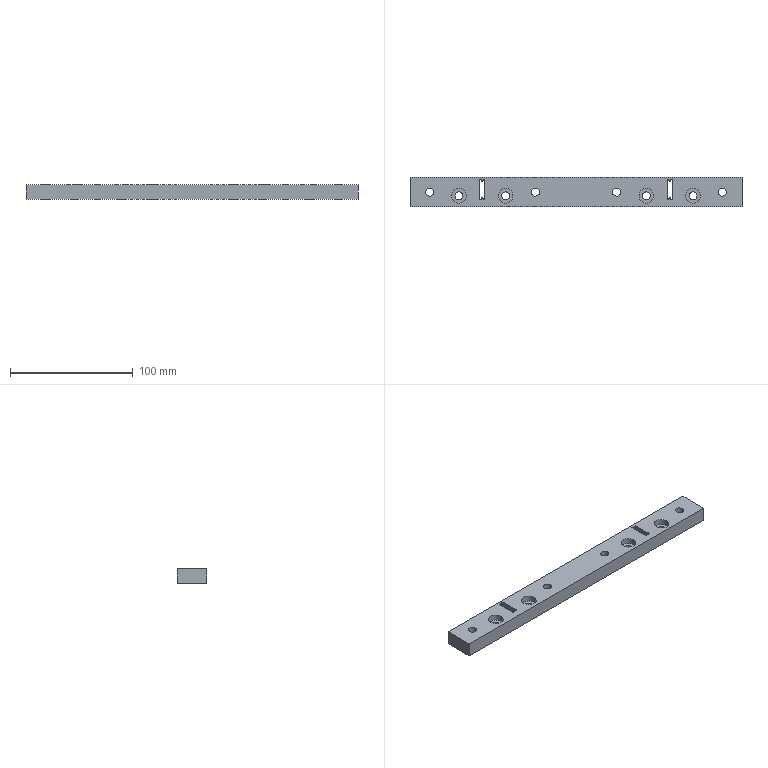Part | STEP file | TAM CHAN PHOI | 1 solid | 74 faces | box 270 x 24 x 12 mm | volume 71324 mm3 | cylinder 44 | plane 30 | commonest cylinder face diameters 0.8 x16 6.4 x8 6.647 x8 12 x8 1.2 x4